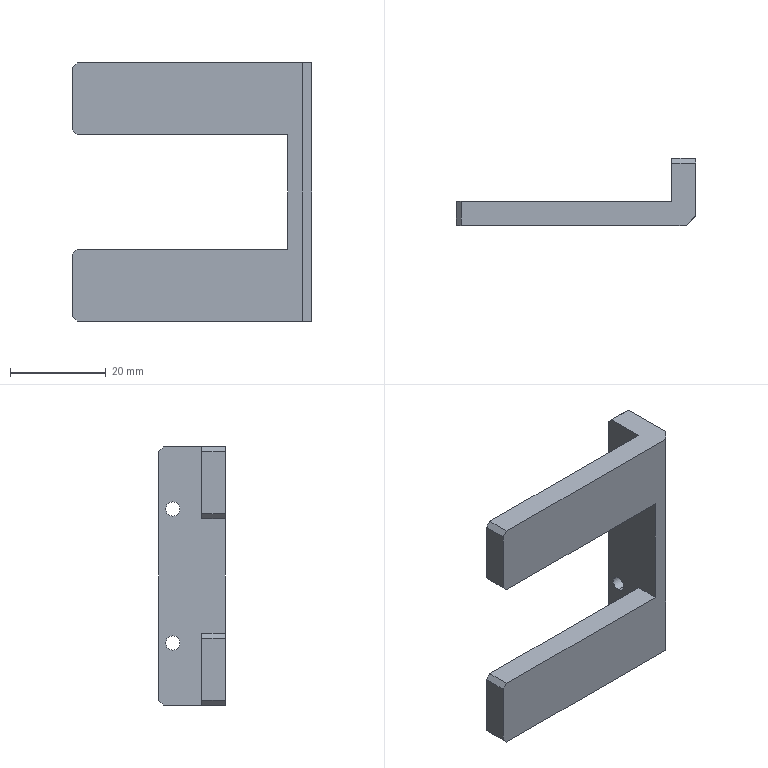Part | STEP file | Guide wheel mechanism revised.sldasm-Part-375 | 1 solid | 23 faces | box 50 x 14 x 54 mm | volume 10336 mm3 | plane 19 | cylinder 4 | commonest cylinder face diameters 3 x4
STEP:
#1=CARTESIAN_POINT('',(0.,11.,12.5));
#2=VERTEX_POINT('',#1);
#3=CARTESIAN_POINT('',(0.,11.,15.5));
#4=VERTEX_POINT('',#3);
#5=CARTESIAN_POINT('',(0.,11.,14.));
#6=DIRECTION('',(-1.,0.,0.));
#7=DIRECTION('',(0.,0.,-1.));
#8=AXIS2_PLACEMENT_3D('',#5,#6,#7);
#9=CIRCLE('',#8,1.5);
#10=EDGE_CURVE('',#2,#4,#9,.T.);
#11=ORIENTED_EDGE('',*,*,#10,.F.);
#12=CARTESIAN_POINT('',(-5.,11.,12.5));
#13=VERTEX_POINT('',#12);
#14=CARTESIAN_POINT('',(0.001,11.,12.5));
#15=DIRECTION('',(-1.,0.,0.));
#16=VECTOR('',#15,1000.);
#17=LINE('',#14,#16);
#18=EDGE_CURVE('',#2,#13,#17,.T.);
#19=ORIENTED_EDGE('',*,*,#18,.T.);
#20=CARTESIAN_POINT('',(-5.,11.,15.5));
#21=VERTEX_POINT('',#20);
#22=CARTESIAN_POINT('',(-5.,11.,14.));
#23=DIRECTION('',(-1.,0.,0.));
#24=DIRECTION('',(0.,0.,1.));
#25=AXIS2_PLACEMENT_3D('',#22,#23,#24);
#26=CIRCLE('',#25,1.5);
#27=EDGE_CURVE('',#13,#21,#26,.T.);
#28=ORIENTED_EDGE('',*,*,#27,.T.);
#29=CARTESIAN_POINT('',(0.001,11.,15.5));
#30=DIRECTION('',(-1.,0.,0.));
#31=VECTOR('',#30,1000.);
#32=LINE('',#29,#31);
#33=EDGE_CURVE('',#4,#21,#32,.T.);
#34=ORIENTED_EDGE('',*,*,#33,.F.);
#35=EDGE_LOOP('',(#11,#19,#28,#34));
#36=FACE_OUTER_BOUND('',#35,.T.);
#37=CARTESIAN_POINT('',(0.001,11.,14.));
#38=DIRECTION('',(-1.,0.,0.));
#39=DIRECTION('',(0.,0.,1.));
#40=AXIS2_PLACEMENT_3D('',#37,#38,#39);
#41=CYLINDRICAL_SURFACE('',#40,1.5);
#42=ADVANCED_FACE('',(#36),#41,.F.);
#43=CARTESIAN_POINT('',(0.,11.,-15.5));
#44=VERTEX_POINT('',#43);
#45=CARTESIAN_POINT('',(0.,11.,-12.5));
#46=VERTEX_POINT('',#45);
#47=CARTESIAN_POINT('',(0.,11.,-14.));
#48=DIRECTION('',(-1.,0.,0.));
#49=DIRECTION('',(0.,0.,-1.));
#50=AXIS2_PLACEMENT_3D('',#47,#48,#49);
#51=CIRCLE('',#50,1.5);
#52=EDGE_CURVE('',#44,#46,#51,.T.);
#53=ORIENTED_EDGE('',*,*,#52,.F.);
#54=CARTESIAN_POINT('',(-5.,11.,-15.5));
#55=VERTEX_POINT('',#54);
#56=CARTESIAN_POINT('',(0.001,11.,-15.5));
#57=DIRECTION('',(-1.,0.,0.));
#58=VECTOR('',#57,1000.);
#59=LINE('',#56,#58);
#60=EDGE_CURVE('',#44,#55,#59,.T.);
#61=ORIENTED_EDGE('',*,*,#60,.T.);
#62=CARTESIAN_POINT('',(-5.,11.,-12.5));
#63=VERTEX_POINT('',#62);
#64=CARTESIAN_POINT('',(-5.,11.,-14.));
#65=DIRECTION('',(-1.,0.,0.));
#66=DIRECTION('',(0.,0.,1.));
#67=AXIS2_PLACEMENT_3D('',#64,#65,#66);
#68=CIRCLE('',#67,1.5);
#69=EDGE_CURVE('',#55,#63,#68,.T.);
#70=ORIENTED_EDGE('',*,*,#69,.T.);
#71=CARTESIAN_POINT('',(0.001,11.,-12.5));
#72=DIRECTION('',(-1.,0.,0.));
#73=VECTOR('',#72,1000.);
#74=LINE('',#71,#73);
#75=EDGE_CURVE('',#46,#63,#74,.T.);
#76=ORIENTED_EDGE('',*,*,#75,.F.);
#77=EDGE_LOOP('',(#53,#61,#70,#76));
#78=FACE_OUTER_BOUND('',#77,.T.);
#79=CARTESIAN_POINT('',(0.001,11.,-14.));
#80=DIRECTION('',(-1.,0.,0.));
#81=DIRECTION('',(0.,0.,1.));
#82=AXIS2_PLACEMENT_3D('',#79,#80,#81);
#83=CYLINDRICAL_SURFACE('',#82,1.5);
#84=ADVANCED_FACE('',(#78),#83,.F.);
#85=CARTESIAN_POINT('',(-50.,0.,-26.));
#86=VERTEX_POINT('',#85);
#87=CARTESIAN_POINT('',(-50.,0.,-13.));
#88=VERTEX_POINT('',#87);
#89=CARTESIAN_POINT('',(-50.,0.,-27.));
#90=DIRECTION('',(0.,0.,1.));
#91=VECTOR('',#90,1000.);
#92=LINE('',#89,#91);
#93=EDGE_CURVE('',#86,#88,#92,.T.);
#94=ORIENTED_EDGE('',*,*,#93,.T.);
#95=CARTESIAN_POINT('',(-50.,5.,-13.));
#96=VERTEX_POINT('',#95);
#97=CARTESIAN_POINT('',(-50.,0.,-13.));
#98=DIRECTION('',(0.,1.,0.));
#99=VECTOR('',#98,1000.);
#100=LINE('',#97,#99);
#101=EDGE_CURVE('',#88,#96,#100,.T.);
#102=ORIENTED_EDGE('',*,*,#101,.T.);
#103=CARTESIAN_POINT('',(-50.,5.,-26.));
#104=VERTEX_POINT('',#103);
#105=CARTESIAN_POINT('',(-50.,5.,-27.));
#106=DIRECTION('',(0.,0.,1.));
#107=VECTOR('',#106,1000.);
#108=LINE('',#105,#107);
#109=EDGE_CURVE('',#104,#96,#108,.T.);
#110=ORIENTED_EDGE('',*,*,#109,.F.);
#111=CARTESIAN_POINT('',(-50.,0.,-26.));
#112=DIRECTION('',(0.,-1.,0.));
#113=VECTOR('',#112,1000.);
#114=LINE('',#111,#113);
#115=EDGE_CURVE('',#104,#86,#114,.T.);
#116=ORIENTED_EDGE('',*,*,#115,.T.);
#117=EDGE_LOOP('',(#94,#102,#110,#116));
#118=FACE_OUTER_BOUND('',#117,.T.);
#119=CARTESIAN_POINT('',(-50.,0.,-27.));
#120=DIRECTION('',(1.,0.,0.));
#121=DIRECTION('',(0.,0.,-1.));
#122=AXIS2_PLACEMENT_3D('',#119,#120,#121);
#123=PLANE('',#122);
#124=ADVANCED_FACE('',(#118),#123,.F.);
#125=ORIENTED_EDGE('',*,*,#109,.T.);
#126=CARTESIAN_POINT('',(-49.,5.,-12.));
#127=VERTEX_POINT('',#126);
#128=CARTESIAN_POINT('',(-50.,5.,-13.));
#129=DIRECTION('',(0.7071,0.,0.7071));
#130=VECTOR('',#129,1000.);
#131=LINE('',#128,#130);
#132=EDGE_CURVE('',#96,#127,#131,.T.);
#133=ORIENTED_EDGE('',*,*,#132,.T.);
#134=CARTESIAN_POINT('',(-5.,5.,-12.));
#135=VERTEX_POINT('',#134);
#136=CARTESIAN_POINT('',(-50.,5.,-12.));
#137=DIRECTION('',(-1.,0.,0.));
#138=VECTOR('',#137,1000.);
#139=LINE('',#136,#138);
#140=EDGE_CURVE('',#135,#127,#139,.T.);
#141=ORIENTED_EDGE('',*,*,#140,.F.);
#142=CARTESIAN_POINT('',(-5.,5.,-27.));
#143=VERTEX_POINT('',#142);
#144=CARTESIAN_POINT('',(-5.,5.,-27.));
#145=DIRECTION('',(0.,0.,1.));
#146=VECTOR('',#145,1000.);
#147=LINE('',#144,#146);
#148=EDGE_CURVE('',#143,#135,#147,.T.);
#149=ORIENTED_EDGE('',*,*,#148,.F.);
#150=CARTESIAN_POINT('',(-49.,5.,-27.));
#151=VERTEX_POINT('',#150);
#152=CARTESIAN_POINT('',(0.,5.,-27.));
#153=DIRECTION('',(1.,0.,0.));
#154=VECTOR('',#153,1000.);
#155=LINE('',#152,#154);
#156=EDGE_CURVE('',#151,#143,#155,.T.);
#157=ORIENTED_EDGE('',*,*,#156,.F.);
#158=CARTESIAN_POINT('',(-49.,5.,-27.));
#159=DIRECTION('',(-0.7071,0.,0.7071));
#160=VECTOR('',#159,1000.);
#161=LINE('',#158,#160);
#162=EDGE_CURVE('',#151,#104,#161,.T.);
#163=ORIENTED_EDGE('',*,*,#162,.T.);
#164=EDGE_LOOP('',(#125,#133,#141,#149,#157,#163));
#165=FACE_OUTER_BOUND('',#164,.T.);
#166=CARTESIAN_POINT('',(0.,5.,-27.));
#167=DIRECTION('',(0.,-1.,0.));
#168=DIRECTION('',(0.,0.,-1.));
#169=AXIS2_PLACEMENT_3D('',#166,#167,#168);
#170=PLANE('',#169);
#171=ADVANCED_FACE('',(#165),#170,.F.);
#172=CARTESIAN_POINT('',(0.,11.,14.));
#173=DIRECTION('',(-1.,0.,0.));
#174=DIRECTION('',(0.,0.,-1.));
#175=AXIS2_PLACEMENT_3D('',#172,#173,#174);
#176=CIRCLE('',#175,1.5);
#177=EDGE_CURVE('',#4,#2,#176,.T.);
#178=ORIENTED_EDGE('',*,*,#177,.T.);
#179=ORIENTED_EDGE('',*,*,#10,.T.);
#180=EDGE_LOOP('',(#178,#179));
#181=FACE_BOUND('',#180,.T.);
#182=CARTESIAN_POINT('',(0.,11.,-14.));
#183=DIRECTION('',(-1.,0.,0.));
#184=DIRECTION('',(0.,0.,-1.));
#185=AXIS2_PLACEMENT_3D('',#182,#183,#184);
#186=CIRCLE('',#185,1.5);
#187=EDGE_CURVE('',#46,#44,#186,.T.);
#188=ORIENTED_EDGE('',*,*,#187,.T.);
#189=ORIENTED_EDGE('',*,*,#52,.T.);
#190=EDGE_LOOP('',(#188,#189));
#191=FACE_BOUND('',#190,.T.);
#192=CARTESIAN_POINT('',(0.,2.,27.));
#193=VERTEX_POINT('',#192);
#194=CARTESIAN_POINT('',(0.,13.,27.));
#195=VERTEX_POINT('',#194);
#196=CARTESIAN_POINT('',(0.,0.,27.));
#197=DIRECTION('',(0.,1.,0.));
#198=VECTOR('',#197,1000.);
#199=LINE('',#196,#198);
#200=EDGE_CURVE('',#193,#195,#199,.T.);
#201=ORIENTED_EDGE('',*,*,#200,.F.);
#202=CARTESIAN_POINT('',(0.,2.,-27.));
#203=VERTEX_POINT('',#202);
#204=CARTESIAN_POINT('',(0.,2.,-27.));
#205=DIRECTION('',(0.,0.,-1.));
#206=VECTOR('',#205,1000.);
#207=LINE('',#204,#206);
#208=EDGE_CURVE('',#193,#203,#207,.T.);
#209=ORIENTED_EDGE('',*,*,#208,.T.);
#210=CARTESIAN_POINT('',(0.,13.,-27.));
#211=VERTEX_POINT('',#210);
#212=CARTESIAN_POINT('',(0.,0.,-27.));
#213=DIRECTION('',(0.,1.,0.));
#214=VECTOR('',#213,1000.);
#215=LINE('',#212,#214);
#216=EDGE_CURVE('',#203,#211,#215,.T.);
#217=ORIENTED_EDGE('',*,*,#216,.T.);
#218=CARTESIAN_POINT('',(0.,14.,-26.));
#219=VERTEX_POINT('',#218);
#220=CARTESIAN_POINT('',(0.,6.5,-33.5));
#221=DIRECTION('',(0.,0.7071,0.7071));
#222=VECTOR('',#221,1000.);
#223=LINE('',#220,#222);
#224=EDGE_CURVE('',#211,#219,#223,.T.);
#225=ORIENTED_EDGE('',*,*,#224,.T.);
#226=CARTESIAN_POINT('',(0.,14.,26.));
#227=VERTEX_POINT('',#226);
#228=CARTESIAN_POINT('',(0.,14.,-27.));
#229=DIRECTION('',(0.,0.,1.));
#230=VECTOR('',#229,1000.);
#231=LINE('',#228,#230);
#232=EDGE_CURVE('',#219,#227,#231,.T.);
#233=ORIENTED_EDGE('',*,*,#232,.T.);
#234=CARTESIAN_POINT('',(0.,33.5,6.5));
#235=DIRECTION('',(0.,-0.7071,0.7071));
#236=VECTOR('',#235,1000.);
#237=LINE('',#234,#236);
#238=EDGE_CURVE('',#227,#195,#237,.T.);
#239=ORIENTED_EDGE('',*,*,#238,.T.);
#240=EDGE_LOOP('',(#201,#209,#217,#225,#233,#239));
#241=FACE_OUTER_BOUND('',#240,.T.);
#242=CARTESIAN_POINT('',(0.,0.,-27.));
#243=DIRECTION('',(1.,0.,0.));
#244=DIRECTION('',(0.,0.,-1.));
#245=AXIS2_PLACEMENT_3D('',#242,#243,#244);
#246=PLANE('',#245);
#247=ADVANCED_FACE('',(#181,#191,#241),#246,.T.);
#248=CARTESIAN_POINT('',(-49.,0.,-27.));
#249=VERTEX_POINT('',#248);
#250=CARTESIAN_POINT('',(-2.,0.,-27.));
#251=VERTEX_POINT('',#250);
#252=CARTESIAN_POINT('',(0.,0.,-27.));
#253=DIRECTION('',(1.,0.,0.));
#254=VECTOR('',#253,1000.);
#255=LINE('',#252,#254);
#256=EDGE_CURVE('',#249,#251,#255,.T.);
#257=ORIENTED_EDGE('',*,*,#256,.T.);
#258=CARTESIAN_POINT('',(-2.,0.,27.));
#259=VERTEX_POINT('',#258);
#260=CARTESIAN_POINT('',(-2.,0.,-27.));
#261=DIRECTION('',(0.,0.,1.));
#262=VECTOR('',#261,1000.);
#263=LINE('',#260,#262);
#264=EDGE_CURVE('',#251,#259,#263,.T.);
#265=ORIENTED_EDGE('',*,*,#264,.T.);
#266=CARTESIAN_POINT('',(-49.,0.,27.));
#267=VERTEX_POINT('',#266);
#268=CARTESIAN_POINT('',(0.,0.,27.));
#269=DIRECTION('',(1.,0.,0.));
#270=VECTOR('',#269,1000.);
#271=LINE('',#268,#270);
#272=EDGE_CURVE('',#267,#259,#271,.T.);
#273=ORIENTED_EDGE('',*,*,#272,.F.);
#274=CARTESIAN_POINT('',(-50.,0.,26.));
#275=VERTEX_POINT('',#274);
#276=CARTESIAN_POINT('',(-51.5,0.,24.5));
#277=DIRECTION('',(-0.7071,0.,-0.7071));
#278=VECTOR('',#277,1000.);
#279=LINE('',#276,#278);
#280=EDGE_CURVE('',#267,#275,#279,.T.);
#281=ORIENTED_EDGE('',*,*,#280,.T.);
#282=CARTESIAN_POINT('',(-50.,0.,13.));
#283=VERTEX_POINT('',#282);
#284=CARTESIAN_POINT('',(-50.,0.,-27.));
#285=DIRECTION('',(0.,0.,1.));
#286=VECTOR('',#285,1000.);
#287=LINE('',#284,#286);
#288=EDGE_CURVE('',#283,#275,#287,.T.);
#289=ORIENTED_EDGE('',*,*,#288,.F.);
#290=CARTESIAN_POINT('',(-49.,0.,12.));
#291=VERTEX_POINT('',#290);
#292=CARTESIAN_POINT('',(-5.,0.,-32.));
#293=DIRECTION('',(0.7071,0.,-0.7071));
#294=VECTOR('',#293,1000.);
#295=LINE('',#292,#294);
#296=EDGE_CURVE('',#283,#291,#295,.T.);
#297=ORIENTED_EDGE('',*,*,#296,.T.);
#298=CARTESIAN_POINT('',(-5.,0.,12.));
#299=VERTEX_POINT('',#298);
#300=CARTESIAN_POINT('',(-50.,0.,12.));
#301=DIRECTION('',(1.,0.,0.));
#302=VECTOR('',#301,1000.);
#303=LINE('',#300,#302);
#304=EDGE_CURVE('',#291,#299,#303,.T.);
#305=ORIENTED_EDGE('',*,*,#304,.T.);
#306=CARTESIAN_POINT('',(-5.,0.,-12.));
#307=VERTEX_POINT('',#306);
#308=CARTESIAN_POINT('',(-5.,0.,-12.));
#309=DIRECTION('',(0.,0.,-1.));
#310=VECTOR('',#309,1000.);
#311=LINE('',#308,#310);
#312=EDGE_CURVE('',#299,#307,#311,.T.);
#313=ORIENTED_EDGE('',*,*,#312,.T.);
#314=CARTESIAN_POINT('',(-49.,0.,-12.));
#315=VERTEX_POINT('',#314);
#316=CARTESIAN_POINT('',(-50.,0.,-12.));
#317=DIRECTION('',(-1.,0.,0.));
#318=VECTOR('',#317,1000.);
#319=LINE('',#316,#318);
#320=EDGE_CURVE('',#307,#315,#319,.T.);
#321=ORIENTED_EDGE('',*,*,#320,.T.);
#322=CARTESIAN_POINT('',(-32.,0.,5.));
#323=DIRECTION('',(-0.7071,0.,-0.7071));
#324=VECTOR('',#323,1000.);
#325=LINE('',#322,#324);
#326=EDGE_CURVE('',#315,#88,#325,.T.);
#327=ORIENTED_EDGE('',*,*,#326,.T.);
#328=ORIENTED_EDGE('',*,*,#93,.F.);
#329=CARTESIAN_POINT('',(-24.5,0.,-51.5));
#330=DIRECTION('',(0.7071,0.,-0.7071));
#331=VECTOR('',#330,1000.);
#332=LINE('',#329,#331);
#333=EDGE_CURVE('',#86,#249,#332,.T.);
#334=ORIENTED_EDGE('',*,*,#333,.T.);
#335=EDGE_LOOP('',(#257,#265,#273,#281,#289,#297,#305,#313,#321,#327,#328,#334));
#336=FACE_OUTER_BOUND('',#335,.T.);
#337=CARTESIAN_POINT('',(0.,0.,-27.));
#338=DIRECTION('',(0.,-1.,0.));
#339=DIRECTION('',(0.,0.,-1.));
#340=AXIS2_PLACEMENT_3D('',#337,#338,#339);
#341=PLANE('',#340);
#342=ADVANCED_FACE('',(#336),#341,.T.);
#343=ORIENTED_EDGE('',*,*,#288,.T.);
#344=CARTESIAN_POINT('',(-50.,5.,26.));
#345=VERTEX_POINT('',#344);
#346=CARTESIAN_POINT('',(-50.,0.,26.));
#347=DIRECTION('',(0.,1.,0.));
#348=VECTOR('',#347,1000.);
#349=LINE('',#346,#348);
#350=EDGE_CURVE('',#275,#345,#349,.T.);
#351=ORIENTED_EDGE('',*,*,#350,.T.);
#352=CARTESIAN_POINT('',(-50.,5.,13.));
#353=VERTEX_POINT('',#352);
#354=CARTESIAN_POINT('',(-50.,5.,-27.));
#355=DIRECTION('',(0.,0.,1.));
#356=VECTOR('',#355,1000.);
#357=LINE('',#354,#356);
#358=EDGE_CURVE('',#353,#345,#357,.T.);
#359=ORIENTED_EDGE('',*,*,#358,.F.);
#360=CARTESIAN_POINT('',(-50.,0.,13.));
#361=DIRECTION('',(0.,-1.,0.));
#362=VECTOR('',#361,1000.);
#363=LINE('',#360,#362);
#364=EDGE_CURVE('',#353,#283,#363,.T.);
#365=ORIENTED_EDGE('',*,*,#364,.T.);
#366=EDGE_LOOP('',(#343,#351,#359,#365));
#367=FACE_OUTER_BOUND('',#366,.T.);
#368=CARTESIAN_POINT('',(-50.,0.,-27.));
#369=DIRECTION('',(1.,0.,0.));
#370=DIRECTION('',(0.,0.,-1.));
#371=AXIS2_PLACEMENT_3D('',#368,#369,#370);
#372=PLANE('',#371);
#373=ADVANCED_FACE('',(#367),#372,.F.);
#374=ORIENTED_EDGE('',*,*,#358,.T.);
#375=CARTESIAN_POINT('',(-49.,5.,27.));
#376=VERTEX_POINT('',#375);
#377=CARTESIAN_POINT('',(-50.,5.,26.));
#378=DIRECTION('',(0.7071,0.,0.7071));
#379=VECTOR('',#378,1000.);
#380=LINE('',#377,#379);
#381=EDGE_CURVE('',#345,#376,#380,.T.);
#382=ORIENTED_EDGE('',*,*,#381,.T.);
#383=CARTESIAN_POINT('',(-5.,5.,27.));
#384=VERTEX_POINT('',#383);
#385=CARTESIAN_POINT('',(0.,5.,27.));
#386=DIRECTION('',(1.,0.,0.));
#387=VECTOR('',#386,1000.);
#388=LINE('',#385,#387);
#389=EDGE_CURVE('',#376,#384,#388,.T.);
#390=ORIENTED_EDGE('',*,*,#389,.T.);
#391=CARTESIAN_POINT('',(-5.,5.,12.));
#392=VERTEX_POINT('',#391);
#393=CARTESIAN_POINT('',(-5.,5.,-27.));
#394=DIRECTION('',(0.,0.,1.));
#395=VECTOR('',#394,1000.);
#396=LINE('',#393,#395);
#397=EDGE_CURVE('',#392,#384,#396,.T.);
#398=ORIENTED_EDGE('',*,*,#397,.F.);
#399=CARTESIAN_POINT('',(-49.,5.,12.));
#400=VERTEX_POINT('',#399);
#401=CARTESIAN_POINT('',(-50.,5.,12.));
#402=DIRECTION('',(1.,0.,0.));
#403=VECTOR('',#402,1000.);
#404=LINE('',#401,#403);
#405=EDGE_CURVE('',#400,#392,#404,.T.);
#406=ORIENTED_EDGE('',*,*,#405,.F.);
#407=CARTESIAN_POINT('',(-49.,5.,12.));
#408=DIRECTION('',(-0.7071,0.,0.7071));
#409=VECTOR('',#408,1000.);
#410=LINE('',#407,#409);
#411=EDGE_CURVE('',#400,#353,#410,.T.);
#412=ORIENTED_EDGE('',*,*,#411,.T.);
#413=EDGE_LOOP('',(#374,#382,#390,#398,#406,#412));
#414=FACE_OUTER_BOUND('',#413,.T.);
#415=CARTESIAN_POINT('',(0.,5.,-27.));
#416=DIRECTION('',(0.,-1.,0.));
#417=DIRECTION('',(0.,0.,-1.));
#418=AXIS2_PLACEMENT_3D('',#415,#416,#417);
#419=PLANE('',#418);
#420=ADVANCED_FACE('',(#414),#419,.F.);
#421=CARTESIAN_POINT('',(-5.,11.,14.));
#422=DIRECTION('',(-1.,0.,0.));
#423=DIRECTION('',(0.,0.,1.));
#424=AXIS2_PLACEMENT_3D('',#421,#422,#423);
#425=CIRCLE('',#424,1.5);
#426=EDGE_CURVE('',#21,#13,#425,.T.);
#427=ORIENTED_EDGE('',*,*,#426,.F.);
#428=ORIENTED_EDGE('',*,*,#27,.F.);
#429=EDGE_LOOP('',(#427,#428));
#430=FACE_BOUND('',#429,.T.);
#431=CARTESIAN_POINT('',(-5.,11.,-14.));
#432=DIRECTION('',(-1.,0.,0.));
#433=DIRECTION('',(0.,0.,1.));
#434=AXIS2_PLACEMENT_3D('',#431,#432,#433);
#435=CIRCLE('',#434,1.5);
#436=EDGE_CURVE('',#63,#55,#435,.T.);
#437=ORIENTED_EDGE('',*,*,#436,.F.);
#438=ORIENTED_EDGE('',*,*,#69,.F.);
#439=EDGE_LOOP('',(#437,#438));
#440=FACE_BOUND('',#439,.T.);
#441=CARTESIAN_POINT('',(-5.,14.,-26.));
#442=VERTEX_POINT('',#441);
#443=CARTESIAN_POINT('',(-5.,14.,26.));
#444=VERTEX_POINT('',#443);
#445=CARTESIAN_POINT('',(-5.,14.,-27.));
#446=DIRECTION('',(0.,0.,1.));
#447=VECTOR('',#446,1000.);
#448=LINE('',#445,#447);
#449=EDGE_CURVE('',#442,#444,#448,.T.);
#450=ORIENTED_EDGE('',*,*,#449,.F.);
#451=CARTESIAN_POINT('',(-5.,13.,-27.));
#452=VERTEX_POINT('',#451);
#453=CARTESIAN_POINT('',(-5.,13.,-27.));
#454=DIRECTION('',(0.,-0.7071,-0.7071));
#455=VECTOR('',#454,1000.);
#456=LINE('',#453,#455);
#457=EDGE_CURVE('',#442,#452,#456,.T.);
#458=ORIENTED_EDGE('',*,*,#457,.T.);
#459=CARTESIAN_POINT('',(-5.,0.,-27.));
#460=DIRECTION('',(0.,1.,0.));
#461=VECTOR('',#460,1000.);
#462=LINE('',#459,#461);
#463=EDGE_CURVE('',#143,#452,#462,.T.);
#464=ORIENTED_EDGE('',*,*,#463,.F.);
#465=ORIENTED_EDGE('',*,*,#148,.T.);
#466=CARTESIAN_POINT('',(-5.,-0.001,-12.));
#467=DIRECTION('',(0.,1.,0.));
#468=VECTOR('',#467,1000.);
#469=LINE('',#466,#468);
#470=EDGE_CURVE('',#307,#135,#469,.T.);
#471=ORIENTED_EDGE('',*,*,#470,.F.);
#472=ORIENTED_EDGE('',*,*,#312,.F.);
#473=CARTESIAN_POINT('',(-5.,-0.001,12.));
#474=DIRECTION('',(0.,1.,0.));
#475=VECTOR('',#474,1000.);
#476=LINE('',#473,#475);
#477=EDGE_CURVE('',#299,#392,#476,.T.);
#478=ORIENTED_EDGE('',*,*,#477,.T.);
#479=ORIENTED_EDGE('',*,*,#397,.T.);
#480=CARTESIAN_POINT('',(-5.,13.,27.));
#481=VERTEX_POINT('',#480);
#482=CARTESIAN_POINT('',(-5.,0.,27.));
#483=DIRECTION('',(0.,1.,0.));
#484=VECTOR('',#483,1000.);
#485=LINE('',#482,#484);
#486=EDGE_CURVE('',#384,#481,#485,.T.);
#487=ORIENTED_EDGE('',*,*,#486,.T.);
#488=CARTESIAN_POINT('',(-5.,14.,26.));
#489=DIRECTION('',(0.,0.7071,-0.7071));
#490=VECTOR('',#489,1000.);
#491=LINE('',#488,#490);
#492=EDGE_CURVE('',#481,#444,#491,.T.);
#493=ORIENTED_EDGE('',*,*,#492,.T.);
#494=EDGE_LOOP('',(#450,#458,#464,#465,#471,#472,#478,#479,#487,#493));
#495=FACE_OUTER_BOUND('',#494,.T.);
#496=CARTESIAN_POINT('',(-5.,0.,-27.));
#497=DIRECTION('',(1.,0.,0.));
#498=DIRECTION('',(0.,0.,-1.));
#499=AXIS2_PLACEMENT_3D('',#496,#497,#498);
#500=PLANE('',#499);
#501=ADVANCED_FACE('',(#430,#440,#495),#500,.F.);
#502=ORIENTED_EDGE('',*,*,#232,.F.);
#503=CARTESIAN_POINT('',(-5.,14.,-26.));
#504=DIRECTION('',(-1.,0.,0.));
#505=VECTOR('',#504,1000.);
#506=LINE('',#503,#505);
#507=EDGE_CURVE('',#219,#442,#506,.T.);
#508=ORIENTED_EDGE('',*,*,#507,.T.);
#509=ORIENTED_EDGE('',*,*,#449,.T.);
#510=CARTESIAN_POINT('',(-5.,14.,26.));
#511=DIRECTION('',(1.,0.,0.));
#512=VECTOR('',#511,1000.);
#513=LINE('',#510,#512);
#514=EDGE_CURVE('',#444,#227,#513,.T.);
#515=ORIENTED_EDGE('',*,*,#514,.T.);
#516=EDGE_LOOP('',(#502,#508,#509,#515));
#517=FACE_OUTER_BOUND('',#516,.T.);
#518=CARTESIAN_POINT('',(-5.,14.,-27.));
#519=DIRECTION('',(0.,-1.,0.));
#520=DIRECTION('',(0.,0.,-1.));
#521=AXIS2_PLACEMENT_3D('',#518,#519,#520);
#522=PLANE('',#521);
#523=ADVANCED_FACE('',(#517),#522,.F.);
#524=ORIENTED_EDGE('',*,*,#216,.F.);
#525=CARTESIAN_POINT('',(-1.,1.,-27.));
#526=DIRECTION('',(-0.7071,-0.7071,0.));
#527=VECTOR('',#526,1000.);
#528=LINE('',#525,#527);
#529=EDGE_CURVE('',#203,#251,#528,.T.);
#530=ORIENTED_EDGE('',*,*,#529,.T.);
#531=ORIENTED_EDGE('',*,*,#256,.F.);
#532=CARTESIAN_POINT('',(-49.,5.,-27.));
#533=DIRECTION('',(0.,1.,0.));
#534=VECTOR('',#533,1000.);
#535=LINE('',#532,#534);
#536=EDGE_CURVE('',#249,#151,#535,.T.);
#537=ORIENTED_EDGE('',*,*,#536,.T.);
#538=ORIENTED_EDGE('',*,*,#156,.T.);
#539=ORIENTED_EDGE('',*,*,#463,.T.);
#540=CARTESIAN_POINT('',(0.,13.,-27.));
#541=DIRECTION('',(1.,0.,0.));
#542=VECTOR('',#541,1000.);
#543=LINE('',#540,#542);
#544=EDGE_CURVE('',#452,#211,#543,.T.);
#545=ORIENTED_EDGE('',*,*,#544,.T.);
#546=EDGE_LOOP('',(#524,#530,#531,#537,#538,#539,#545));
#547=FACE_OUTER_BOUND('',#546,.T.);
#548=CARTESIAN_POINT('',(0.,0.,-27.));
#549=DIRECTION('',(0.,0.,-1.));
#550=DIRECTION('',(-1.,0.,0.));
#551=AXIS2_PLACEMENT_3D('',#548,#549,#550);
#552=PLANE('',#551);
#553=ADVANCED_FACE('',(#547),#552,.T.);
#554=ORIENTED_EDGE('',*,*,#272,.T.);
#555=CARTESIAN_POINT('',(-2.,0.,27.));
#556=DIRECTION('',(0.7071,0.7071,0.));
#557=VECTOR('',#556,1000.);
#558=LINE('',#555,#557);
#559=EDGE_CURVE('',#259,#193,#558,.T.);
#560=ORIENTED_EDGE('',*,*,#559,.T.);
#561=ORIENTED_EDGE('',*,*,#200,.T.);
#562=CARTESIAN_POINT('',(0.,13.,27.));
#563=DIRECTION('',(-1.,0.,0.));
#564=VECTOR('',#563,1000.);
#565=LINE('',#562,#564);
#566=EDGE_CURVE('',#195,#481,#565,.T.);
#567=ORIENTED_EDGE('',*,*,#566,.T.);
#568=ORIENTED_EDGE('',*,*,#486,.F.);
#569=ORIENTED_EDGE('',*,*,#389,.F.);
#570=CARTESIAN_POINT('',(-49.,0.,27.));
#571=DIRECTION('',(0.,-1.,0.));
#572=VECTOR('',#571,1000.);
#573=LINE('',#570,#572);
#574=EDGE_CURVE('',#376,#267,#573,.T.);
#575=ORIENTED_EDGE('',*,*,#574,.T.);
#576=EDGE_LOOP('',(#554,#560,#561,#567,#568,#569,#575));
#577=FACE_OUTER_BOUND('',#576,.T.);
#578=CARTESIAN_POINT('',(0.,0.,27.));
#579=DIRECTION('',(0.,0.,-1.));
#580=DIRECTION('',(-1.,0.,0.));
#581=AXIS2_PLACEMENT_3D('',#578,#579,#580);
#582=PLANE('',#581);
#583=ADVANCED_FACE('',(#577),#582,.F.);
#584=ORIENTED_EDGE('',*,*,#140,.T.);
#585=CARTESIAN_POINT('',(-49.,-0.001,-12.));
#586=DIRECTION('',(0.,-1.,0.));
#587=VECTOR('',#586,1000.);
#588=LINE('',#585,#587);
#589=EDGE_CURVE('',#127,#315,#588,.T.);
#590=ORIENTED_EDGE('',*,*,#589,.T.);
#591=ORIENTED_EDGE('',*,*,#320,.F.);
#592=ORIENTED_EDGE('',*,*,#470,.T.);
#593=EDGE_LOOP('',(#584,#590,#591,#592));
#594=FACE_OUTER_BOUND('',#593,.T.);
#595=CARTESIAN_POINT('',(-50.,-0.001,-12.));
#596=DIRECTION('',(0.,0.,-1.));
#597=DIRECTION('',(-1.,0.,0.));
#598=AXIS2_PLACEMENT_3D('',#595,#596,#597);
#599=PLANE('',#598);
#600=ADVANCED_FACE('',(#594),#599,.F.);
#601=ORIENTED_EDGE('',*,*,#304,.F.);
#602=CARTESIAN_POINT('',(-49.,-0.001,12.));
#603=DIRECTION('',(0.,1.,0.));
#604=VECTOR('',#603,1000.);
#605=LINE('',#602,#604);
#606=EDGE_CURVE('',#291,#400,#605,.T.);
#607=ORIENTED_EDGE('',*,*,#606,.T.);
#608=ORIENTED_EDGE('',*,*,#405,.T.);
#609=ORIENTED_EDGE('',*,*,#477,.F.);
#610=EDGE_LOOP('',(#601,#607,#608,#609));
#611=FACE_OUTER_BOUND('',#610,.T.);
#612=CARTESIAN_POINT('',(-50.,-0.001,12.));
#613=DIRECTION('',(0.,0.,1.));
#614=DIRECTION('',(1.,0.,0.));
#615=AXIS2_PLACEMENT_3D('',#612,#613,#614);
#616=PLANE('',#615);
#617=ADVANCED_FACE('',(#611),#616,.F.);
#618=ORIENTED_EDGE('',*,*,#60,.F.);
#619=ORIENTED_EDGE('',*,*,#187,.F.);
#620=ORIENTED_EDGE('',*,*,#75,.T.);
#621=ORIENTED_EDGE('',*,*,#436,.T.);
#622=EDGE_LOOP('',(#618,#619,#620,#621));
#623=FACE_OUTER_BOUND('',#622,.T.);
#624=CARTESIAN_POINT('',(0.001,11.,-14.));
#625=DIRECTION('',(-1.,0.,0.));
#626=DIRECTION('',(0.,0.,1.));
#627=AXIS2_PLACEMENT_3D('',#624,#625,#626);
#628=CYLINDRICAL_SURFACE('',#627,1.5);
#629=ADVANCED_FACE('',(#623),#628,.F.);
#630=ORIENTED_EDGE('',*,*,#18,.F.);
#631=ORIENTED_EDGE('',*,*,#177,.F.);
#632=ORIENTED_EDGE('',*,*,#33,.T.);
#633=ORIENTED_EDGE('',*,*,#426,.T.);
#634=EDGE_LOOP('',(#630,#631,#632,#633));
#635=FACE_OUTER_BOUND('',#634,.T.);
#636=CARTESIAN_POINT('',(0.001,11.,14.));
#637=DIRECTION('',(-1.,0.,0.));
#638=DIRECTION('',(0.,0.,1.));
#639=AXIS2_PLACEMENT_3D('',#636,#637,#638);
#640=CYLINDRICAL_SURFACE('',#639,1.5);
#641=ADVANCED_FACE('',(#635),#640,.F.);
#642=ORIENTED_EDGE('',*,*,#280,.F.);
#643=ORIENTED_EDGE('',*,*,#574,.F.);
#644=ORIENTED_EDGE('',*,*,#381,.F.);
#645=ORIENTED_EDGE('',*,*,#350,.F.);
#646=EDGE_LOOP('',(#642,#643,#644,#645));
#647=FACE_OUTER_BOUND('',#646,.T.);
#648=CARTESIAN_POINT('',(-50.,0.,26.));
#649=DIRECTION('',(0.7071,0.,-0.7071));
#650=DIRECTION('',(0.,1.,0.));
#651=AXIS2_PLACEMENT_3D('',#648,#649,#650);
#652=PLANE('',#651);
#653=ADVANCED_FACE('',(#647),#652,.F.);
#654=ORIENTED_EDGE('',*,*,#296,.F.);
#655=ORIENTED_EDGE('',*,*,#364,.F.);
#656=ORIENTED_EDGE('',*,*,#411,.F.);
#657=ORIENTED_EDGE('',*,*,#606,.F.);
#658=EDGE_LOOP('',(#654,#655,#656,#657));
#659=FACE_OUTER_BOUND('',#658,.T.);
#660=CARTESIAN_POINT('',(-49.,-0.001,12.));
#661=DIRECTION('',(0.7071,0.,0.7071));
#662=DIRECTION('',(0.,1.,0.));
#663=AXIS2_PLACEMENT_3D('',#660,#661,#662);
#664=PLANE('',#663);
#665=ADVANCED_FACE('',(#659),#664,.F.);
#666=ORIENTED_EDGE('',*,*,#326,.F.);
#667=ORIENTED_EDGE('',*,*,#589,.F.);
#668=ORIENTED_EDGE('',*,*,#132,.F.);
#669=ORIENTED_EDGE('',*,*,#101,.F.);
#670=EDGE_LOOP('',(#666,#667,#668,#669));
#671=FACE_OUTER_BOUND('',#670,.T.);
#672=CARTESIAN_POINT('',(-50.,0.,-13.));
#673=DIRECTION('',(0.7071,0.,-0.7071));
#674=DIRECTION('',(0.,1.,0.));
#675=AXIS2_PLACEMENT_3D('',#672,#673,#674);
#676=PLANE('',#675);
#677=ADVANCED_FACE('',(#671),#676,.F.);
#678=ORIENTED_EDGE('',*,*,#333,.F.);
#679=ORIENTED_EDGE('',*,*,#115,.F.);
#680=ORIENTED_EDGE('',*,*,#162,.F.);
#681=ORIENTED_EDGE('',*,*,#536,.F.);
#682=EDGE_LOOP('',(#678,#679,#680,#681));
#683=FACE_OUTER_BOUND('',#682,.T.);
#684=CARTESIAN_POINT('',(-49.,0.,-27.));
#685=DIRECTION('',(-0.7071,0.,-0.7071));
#686=DIRECTION('',(0.,-1.,0.));
#687=AXIS2_PLACEMENT_3D('',#684,#685,#686);
#688=PLANE('',#687);
#689=ADVANCED_FACE('',(#683),#688,.T.);
#690=ORIENTED_EDGE('',*,*,#457,.F.);
#691=ORIENTED_EDGE('',*,*,#507,.F.);
#692=ORIENTED_EDGE('',*,*,#224,.F.);
#693=ORIENTED_EDGE('',*,*,#544,.F.);
#694=EDGE_LOOP('',(#690,#691,#692,#693));
#695=FACE_OUTER_BOUND('',#694,.T.);
#696=CARTESIAN_POINT('',(0.,13.,-27.));
#697=DIRECTION('',(0.,0.7071,-0.7071));
#698=DIRECTION('',(-1.,0.,0.));
#699=AXIS2_PLACEMENT_3D('',#696,#697,#698);
#700=PLANE('',#699);
#701=ADVANCED_FACE('',(#695),#700,.T.);
#702=ORIENTED_EDGE('',*,*,#492,.F.);
#703=ORIENTED_EDGE('',*,*,#566,.F.);
#704=ORIENTED_EDGE('',*,*,#238,.F.);
#705=ORIENTED_EDGE('',*,*,#514,.F.);
#706=EDGE_LOOP('',(#702,#703,#704,#705));
#707=FACE_OUTER_BOUND('',#706,.T.);
#708=CARTESIAN_POINT('',(-5.,14.,26.));
#709=DIRECTION('',(0.,-0.7071,-0.7071));
#710=DIRECTION('',(1.,0.,0.));
#711=AXIS2_PLACEMENT_3D('',#708,#709,#710);
#712=PLANE('',#711);
#713=ADVANCED_FACE('',(#707),#712,.F.);
#714=ORIENTED_EDGE('',*,*,#529,.F.);
#715=ORIENTED_EDGE('',*,*,#208,.F.);
#716=ORIENTED_EDGE('',*,*,#559,.F.);
#717=ORIENTED_EDGE('',*,*,#264,.F.);
#718=EDGE_LOOP('',(#714,#715,#716,#717));
#719=FACE_OUTER_BOUND('',#718,.T.);
#720=CARTESIAN_POINT('',(-2.,0.,-27.));
#721=DIRECTION('',(-0.7071,0.7071,0.));
#722=DIRECTION('',(0.,0.,1.));
#723=AXIS2_PLACEMENT_3D('',#720,#721,#722);
#724=PLANE('',#723);
#725=ADVANCED_FACE('',(#719),#724,.F.);
#726=CLOSED_SHELL('',(#42,#84,#124,#171,#247,#342,#373,#420,#501,#523,#553,#583,#600,#617,#629,#641,#653,#665,#677,#689,#701,#713,#725));
#727=MANIFOLD_SOLID_BREP('',#726);
#728=CARTESIAN_POINT('',(0.,0.,0.));
#729=DIRECTION('',(0.,0.,1.));
#730=DIRECTION('',(1.,0.,0.));
#731=AXIS2_PLACEMENT_3D('',#728,#729,#730);
#732=(LENGTH_UNIT()NAMED_UNIT(*)SI_UNIT(.MILLI.,.METRE.));
#733=UNCERTAINTY_MEASURE_WITH_UNIT(LENGTH_MEASURE(0.00001),#732,'','');
#734=(NAMED_UNIT(*)PLANE_ANGLE_UNIT()SI_UNIT($,.RADIAN.));
#735=(NAMED_UNIT(*)SI_UNIT($,.STERADIAN.)SOLID_ANGLE_UNIT());
#736=(GEOMETRIC_REPRESENTATION_CONTEXT(3)GLOBAL_UNCERTAINTY_ASSIGNED_CONTEXT((#733))GLOBAL_UNIT_ASSIGNED_CONTEXT((#732,#734,#735))REPRESENTATION_CONTEXT('',''));
#737=ADVANCED_BREP_SHAPE_REPRESENTATION('',(#727,#731),#736);